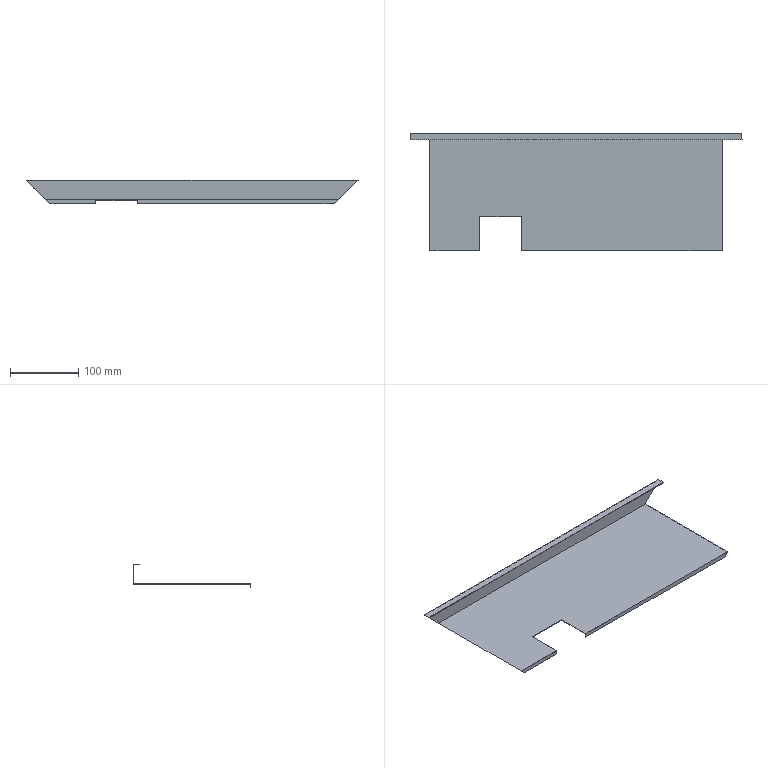Part | STEP file | 09-07 Inner side plate 4 | 1 solid | 18 faces | box 485 x 172 x 35 mm | volume 89624 mm3 | plane 18
STEP:
#1=CARTESIAN_POINT('',(0.,0.,0.));
#2=DIRECTION('',(0.,0.,1.));
#3=DIRECTION('',(1.,0.,0.));
#4=AXIS2_PLACEMENT_3D('',#1,#2,#3);
#5=CARTESIAN_POINT('',(162.5,50.,1.));
#6=VERTEX_POINT('',#5);
#7=CARTESIAN_POINT('',(102.,50.,1.));
#8=VERTEX_POINT('',#7);
#9=CARTESIAN_POINT('',(242.5,50.,1.));
#10=DIRECTION('',(-1.,0.,0.));
#11=VECTOR('',#10,1.);
#12=LINE('',#9,#11);
#13=CARTESIAN_POINT('',(29.,0.,1.));
#14=DIRECTION('',(0.,0.,-1.));
#15=DIRECTION('',(0.,1.,0.));
#16=AXIS2_PLACEMENT_3D('',#13,#14,#15);
#17=PLANE('',#16);
#18=CARTESIAN_POINT('',(50.,213.5));
#19=DIRECTION('',(0.,-1.));
#20=VECTOR('',#19,1.);
#21=LINE('',#18,#20);
#22=(GEOMETRIC_REPRESENTATION_CONTEXT(2)PARAMETRIC_REPRESENTATION_CONTEXT()REPRESENTATION_CONTEXT('',''));
#23=DEFINITIONAL_REPRESENTATION('',(#21),#22);
#24=PCURVE('',#17,#23);
#25=CARTESIAN_POINT('',(102.,50.,1.));
#26=DIRECTION('',(0.,-1.,0.));
#27=DIRECTION('',(0.,0.,-1.));
#28=AXIS2_PLACEMENT_3D('',#25,#26,#27);
#29=PLANE('',#28);
#30=CARTESIAN_POINT('',(0.,140.5));
#31=DIRECTION('',(0.,-1.));
#32=VECTOR('',#31,1.);
#33=LINE('',#30,#32);
#34=(GEOMETRIC_REPRESENTATION_CONTEXT(2)PARAMETRIC_REPRESENTATION_CONTEXT()REPRESENTATION_CONTEXT('',''));
#35=DEFINITIONAL_REPRESENTATION('',(#33),#34);
#36=PCURVE('',#29,#35);
#37=SURFACE_CURVE('',#12,(#24,#36),.PCURVE_S1.);
#38=EDGE_CURVE('',#6,#8,#37,.T.);
#39=ORIENTED_EDGE('',*,*,#38,.F.);
#40=CARTESIAN_POINT('',(162.5,0.,1.));
#41=VERTEX_POINT('',#40);
#42=CARTESIAN_POINT('',(162.5,85.5,1.));
#43=DIRECTION('',(0.,1.,0.));
#44=VECTOR('',#43,1.);
#45=LINE('',#42,#44);
#46=CARTESIAN_POINT('',(85.5,133.5));
#47=DIRECTION('',(1.,0.));
#48=VECTOR('',#47,1.);
#49=LINE('',#46,#48);
#50=(GEOMETRIC_REPRESENTATION_CONTEXT(2)PARAMETRIC_REPRESENTATION_CONTEXT()REPRESENTATION_CONTEXT('',''));
#51=DEFINITIONAL_REPRESENTATION('',(#49),#50);
#52=PCURVE('',#17,#51);
#53=CARTESIAN_POINT('',(162.5,0.,-5.));
#54=DIRECTION('',(-1.,0.,0.));
#55=DIRECTION('',(0.,0.,1.));
#56=AXIS2_PLACEMENT_3D('',#53,#54,#55);
#57=PLANE('',#56);
#58=CARTESIAN_POINT('',(6.,85.5));
#59=DIRECTION('',(0.,1.));
#60=VECTOR('',#59,1.);
#61=LINE('',#58,#60);
#62=(GEOMETRIC_REPRESENTATION_CONTEXT(2)PARAMETRIC_REPRESENTATION_CONTEXT()REPRESENTATION_CONTEXT('',''));
#63=DEFINITIONAL_REPRESENTATION('',(#61),#62);
#64=PCURVE('',#57,#63);
#65=SURFACE_CURVE('',#45,(#52,#64),.PCURVE_S1.);
#66=EDGE_CURVE('',#41,#6,#65,.T.);
#67=ORIENTED_EDGE('',*,*,#66,.F.);
#68=CARTESIAN_POINT('',(456.,0.,1.));
#69=VERTEX_POINT('',#68);
#70=CARTESIAN_POINT('',(242.5,0.,1.));
#71=DIRECTION('',(-1.,0.,0.));
#72=VECTOR('',#71,1.);
#73=LINE('',#70,#72);
#74=CARTESIAN_POINT('',(0.,213.5));
#75=DIRECTION('',(0.,-1.));
#76=VECTOR('',#75,1.);
#77=LINE('',#74,#76);
#78=(GEOMETRIC_REPRESENTATION_CONTEXT(2)PARAMETRIC_REPRESENTATION_CONTEXT()REPRESENTATION_CONTEXT('',''));
#79=DEFINITIONAL_REPRESENTATION('',(#77),#78);
#80=PCURVE('',#17,#79);
#81=CARTESIAN_POINT('',(162.5,0.,-5.));
#82=DIRECTION('',(0.,1.,0.));
#83=DIRECTION('',(0.,0.,1.));
#84=AXIS2_PLACEMENT_3D('',#81,#82,#83);
#85=PLANE('',#84);
#86=CARTESIAN_POINT('',(6.,80.));
#87=DIRECTION('',(0.,-1.));
#88=VECTOR('',#87,1.);
#89=LINE('',#86,#88);
#90=(GEOMETRIC_REPRESENTATION_CONTEXT(2)PARAMETRIC_REPRESENTATION_CONTEXT()REPRESENTATION_CONTEXT('',''));
#91=DEFINITIONAL_REPRESENTATION('',(#89),#90);
#92=PCURVE('',#85,#91);
#93=SURFACE_CURVE('',#73,(#80,#92),.PCURVE_S1.);
#94=EDGE_CURVE('',#69,#41,#93,.T.);
#95=ORIENTED_EDGE('',*,*,#94,.F.);
#96=CARTESIAN_POINT('',(456.,171.,1.));
#97=VERTEX_POINT('',#96);
#98=CARTESIAN_POINT('',(456.,85.5,1.));
#99=DIRECTION('',(0.,-1.,0.));
#100=VECTOR('',#99,1.);
#101=LINE('',#98,#100);
#102=CARTESIAN_POINT('',(85.5,427.));
#103=DIRECTION('',(-1.,0.));
#104=VECTOR('',#103,1.);
#105=LINE('',#102,#104);
#106=(GEOMETRIC_REPRESENTATION_CONTEXT(2)PARAMETRIC_REPRESENTATION_CONTEXT()REPRESENTATION_CONTEXT('',''));
#107=DEFINITIONAL_REPRESENTATION('',(#105),#106);
#108=PCURVE('',#17,#107);
#109=CARTESIAN_POINT('',(450.,0.,-5.));
#110=DIRECTION('',(-0.7071,0.,0.7071));
#111=DIRECTION('',(0.7071,0.,0.7071));
#112=AXIS2_PLACEMENT_3D('',#109,#110,#111);
#113=PLANE('',#112);
#114=CARTESIAN_POINT('',(8.485,85.5));
#115=DIRECTION('',(0.,-1.));
#116=VECTOR('',#115,1.);
#117=LINE('',#114,#116);
#118=(GEOMETRIC_REPRESENTATION_CONTEXT(2)PARAMETRIC_REPRESENTATION_CONTEXT()REPRESENTATION_CONTEXT('',''));
#119=DEFINITIONAL_REPRESENTATION('',(#117),#118);
#120=PCURVE('',#113,#119);
#121=SURFACE_CURVE('',#101,(#108,#120),.PCURVE_S1.);
#122=EDGE_CURVE('',#97,#69,#121,.T.);
#123=ORIENTED_EDGE('',*,*,#122,.F.);
#124=CARTESIAN_POINT('',(29.,171.,1.));
#125=VERTEX_POINT('',#124);
#126=CARTESIAN_POINT('',(242.5,171.,1.));
#127=DIRECTION('',(1.,0.,0.));
#128=VECTOR('',#127,1.);
#129=LINE('',#126,#128);
#130=CARTESIAN_POINT('',(171.,213.5));
#131=DIRECTION('',(0.,1.));
#132=VECTOR('',#131,1.);
#133=LINE('',#130,#132);
#134=(GEOMETRIC_REPRESENTATION_CONTEXT(2)PARAMETRIC_REPRESENTATION_CONTEXT()REPRESENTATION_CONTEXT('',''));
#135=DEFINITIONAL_REPRESENTATION('',(#133),#134);
#136=PCURVE('',#17,#135);
#137=CARTESIAN_POINT('',(-1.898,171.,1.));
#138=DIRECTION('',(0.,1.,0.));
#139=DIRECTION('',(0.,0.,1.));
#140=AXIS2_PLACEMENT_3D('',#137,#138,#139);
#141=PLANE('',#140);
#142=CARTESIAN_POINT('',(0.,244.398));
#143=DIRECTION('',(0.,1.));
#144=VECTOR('',#143,1.);
#145=LINE('',#142,#144);
#146=(GEOMETRIC_REPRESENTATION_CONTEXT(2)PARAMETRIC_REPRESENTATION_CONTEXT()REPRESENTATION_CONTEXT('',''));
#147=DEFINITIONAL_REPRESENTATION('',(#145),#146);
#148=PCURVE('',#141,#147);
#149=SURFACE_CURVE('',#129,(#136,#148),.PCURVE_S1.);
#150=EDGE_CURVE('',#125,#97,#149,.T.);
#151=ORIENTED_EDGE('',*,*,#150,.F.);
#152=CARTESIAN_POINT('',(29.,0.,1.));
#153=VERTEX_POINT('',#152);
#154=CARTESIAN_POINT('',(29.,85.5,1.));
#155=DIRECTION('',(0.,1.,0.));
#156=VECTOR('',#155,1.);
#157=LINE('',#154,#156);
#158=CARTESIAN_POINT('',(85.5,0.));
#159=DIRECTION('',(1.,0.));
#160=VECTOR('',#159,1.);
#161=LINE('',#158,#160);
#162=(GEOMETRIC_REPRESENTATION_CONTEXT(2)PARAMETRIC_REPRESENTATION_CONTEXT()REPRESENTATION_CONTEXT('',''));
#163=DEFINITIONAL_REPRESENTATION('',(#161),#162);
#164=PCURVE('',#17,#163);
#165=CARTESIAN_POINT('',(0.,0.,30.));
#166=DIRECTION('',(0.7071,0.,0.7071));
#167=DIRECTION('',(0.7071,0.,-0.7071));
#168=AXIS2_PLACEMENT_3D('',#165,#166,#167);
#169=PLANE('',#168);
#170=CARTESIAN_POINT('',(41.012,85.5));
#171=DIRECTION('',(0.,1.));
#172=VECTOR('',#171,1.);
#173=LINE('',#170,#172);
#174=(GEOMETRIC_REPRESENTATION_CONTEXT(2)PARAMETRIC_REPRESENTATION_CONTEXT()REPRESENTATION_CONTEXT('',''));
#175=DEFINITIONAL_REPRESENTATION('',(#173),#174);
#176=PCURVE('',#169,#175);
#177=SURFACE_CURVE('',#157,(#164,#176),.PCURVE_S1.);
#178=EDGE_CURVE('',#153,#125,#177,.T.);
#179=ORIENTED_EDGE('',*,*,#178,.F.);
#180=CARTESIAN_POINT('',(102.,0.,1.));
#181=VERTEX_POINT('',#180);
#182=CARTESIAN_POINT('',(242.5,0.,1.));
#183=DIRECTION('',(-1.,0.,0.));
#184=VECTOR('',#183,1.);
#185=LINE('',#182,#184);
#186=CARTESIAN_POINT('',(0.,213.5));
#187=DIRECTION('',(0.,-1.));
#188=VECTOR('',#187,1.);
#189=LINE('',#186,#188);
#190=(GEOMETRIC_REPRESENTATION_CONTEXT(2)PARAMETRIC_REPRESENTATION_CONTEXT()REPRESENTATION_CONTEXT('',''));
#191=DEFINITIONAL_REPRESENTATION('',(#189),#190);
#192=PCURVE('',#17,#191);
#193=CARTESIAN_POINT('',(28.562,0.,-5.));
#194=DIRECTION('',(0.,1.,0.));
#195=DIRECTION('',(0.,0.,1.));
#196=AXIS2_PLACEMENT_3D('',#193,#194,#195);
#197=PLANE('',#196);
#198=CARTESIAN_POINT('',(6.,213.938));
#199=DIRECTION('',(0.,-1.));
#200=VECTOR('',#199,1.);
#201=LINE('',#198,#200);
#202=(GEOMETRIC_REPRESENTATION_CONTEXT(2)PARAMETRIC_REPRESENTATION_CONTEXT()REPRESENTATION_CONTEXT('',''));
#203=DEFINITIONAL_REPRESENTATION('',(#201),#202);
#204=PCURVE('',#197,#203);
#205=SURFACE_CURVE('',#185,(#192,#204),.PCURVE_S1.);
#206=EDGE_CURVE('',#181,#153,#205,.T.);
#207=ORIENTED_EDGE('',*,*,#206,.F.);
#208=CARTESIAN_POINT('',(102.,85.5,1.));
#209=DIRECTION('',(0.,-1.,0.));
#210=VECTOR('',#209,1.);
#211=LINE('',#208,#210);
#212=CARTESIAN_POINT('',(85.5,73.));
#213=DIRECTION('',(-1.,0.));
#214=VECTOR('',#213,1.);
#215=LINE('',#212,#214);
#216=(GEOMETRIC_REPRESENTATION_CONTEXT(2)PARAMETRIC_REPRESENTATION_CONTEXT()REPRESENTATION_CONTEXT('',''));
#217=DEFINITIONAL_REPRESENTATION('',(#215),#216);
#218=PCURVE('',#17,#217);
#219=CARTESIAN_POINT('',(102.,0.,-5.));
#220=DIRECTION('',(1.,0.,0.));
#221=DIRECTION('',(0.,1.,0.));
#222=AXIS2_PLACEMENT_3D('',#219,#220,#221);
#223=PLANE('',#222);
#224=CARTESIAN_POINT('',(85.5,6.));
#225=DIRECTION('',(-1.,0.));
#226=VECTOR('',#225,1.);
#227=LINE('',#224,#226);
#228=(GEOMETRIC_REPRESENTATION_CONTEXT(2)PARAMETRIC_REPRESENTATION_CONTEXT()REPRESENTATION_CONTEXT('',''));
#229=DEFINITIONAL_REPRESENTATION('',(#227),#228);
#230=PCURVE('',#223,#229);
#231=SURFACE_CURVE('',#211,(#218,#230),.PCURVE_S1.);
#232=EDGE_CURVE('',#8,#181,#231,.T.);
#233=ORIENTED_EDGE('',*,*,#232,.F.);
#234=EDGE_LOOP('',(#39,#67,#95,#123,#151,#179,#207,#233));
#235=FACE_BOUND('',#234,.T.);
#236=ADVANCED_FACE('',(#235),#17,.F.);
#237=CARTESIAN_POINT('',(102.,1.,-0.000000001));
#238=VERTEX_POINT('',#237);
#239=CARTESIAN_POINT('',(102.,50.,-0.000000001));
#240=VERTEX_POINT('',#239);
#241=CARTESIAN_POINT('',(102.,25.,-0.000000002));
#242=DIRECTION('',(0.,1.,0.));
#243=VECTOR('',#242,1.);
#244=LINE('',#241,#243);
#245=CARTESIAN_POINT('',(25.,5.));
#246=DIRECTION('',(1.,0.));
#247=VECTOR('',#246,1.);
#248=LINE('',#245,#247);
#249=(GEOMETRIC_REPRESENTATION_CONTEXT(2)PARAMETRIC_REPRESENTATION_CONTEXT()REPRESENTATION_CONTEXT('',''));
#250=DEFINITIONAL_REPRESENTATION('',(#248),#249);
#251=PCURVE('',#223,#250);
#252=CARTESIAN_POINT('',(30.,172.,0.));
#253=DIRECTION('',(0.,0.,1.));
#254=DIRECTION('',(0.,-1.,0.));
#255=AXIS2_PLACEMENT_3D('',#252,#253,#254);
#256=PLANE('',#255);
#257=CARTESIAN_POINT('',(147.,72.));
#258=DIRECTION('',(-1.,0.));
#259=VECTOR('',#258,1.);
#260=LINE('',#257,#259);
#261=(GEOMETRIC_REPRESENTATION_CONTEXT(2)PARAMETRIC_REPRESENTATION_CONTEXT()REPRESENTATION_CONTEXT('',''));
#262=DEFINITIONAL_REPRESENTATION('',(#260),#261);
#263=PCURVE('',#256,#262);
#264=SURFACE_CURVE('',#244,(#251,#263),.PCURVE_S1.);
#265=EDGE_CURVE('',#238,#240,#264,.T.);
#266=ORIENTED_EDGE('',*,*,#265,.T.);
#267=CARTESIAN_POINT('',(102.,50.,-2.));
#268=DIRECTION('',(0.,0.,1.));
#269=VECTOR('',#268,1.);
#270=LINE('',#267,#269);
#271=CARTESIAN_POINT('',(50.,3.));
#272=DIRECTION('',(0.,1.));
#273=VECTOR('',#272,1.);
#274=LINE('',#271,#273);
#275=(GEOMETRIC_REPRESENTATION_CONTEXT(2)PARAMETRIC_REPRESENTATION_CONTEXT()REPRESENTATION_CONTEXT('',''));
#276=DEFINITIONAL_REPRESENTATION('',(#274),#275);
#277=PCURVE('',#223,#276);
#278=CARTESIAN_POINT('',(3.,0.));
#279=DIRECTION('',(-1.,0.));
#280=VECTOR('',#279,1.);
#281=LINE('',#278,#280);
#282=(GEOMETRIC_REPRESENTATION_CONTEXT(2)PARAMETRIC_REPRESENTATION_CONTEXT()REPRESENTATION_CONTEXT('',''));
#283=DEFINITIONAL_REPRESENTATION('',(#281),#282);
#284=PCURVE('',#29,#283);
#285=SURFACE_CURVE('',#270,(#277,#284),.PCURVE_S1.);
#286=EDGE_CURVE('',#240,#8,#285,.T.);
#287=ORIENTED_EDGE('',*,*,#286,.T.);
#288=ORIENTED_EDGE('',*,*,#232,.T.);
#289=CARTESIAN_POINT('',(102.,0.,-5.));
#290=VERTEX_POINT('',#289);
#291=CARTESIAN_POINT('',(102.,0.,-2.));
#292=DIRECTION('',(0.,0.,-1.));
#293=VECTOR('',#292,1.);
#294=LINE('',#291,#293);
#295=CARTESIAN_POINT('',(0.,3.));
#296=DIRECTION('',(0.,-1.));
#297=VECTOR('',#296,1.);
#298=LINE('',#295,#297);
#299=(GEOMETRIC_REPRESENTATION_CONTEXT(2)PARAMETRIC_REPRESENTATION_CONTEXT()REPRESENTATION_CONTEXT('',''));
#300=DEFINITIONAL_REPRESENTATION('',(#298),#299);
#301=PCURVE('',#223,#300);
#302=CARTESIAN_POINT('',(3.,73.438));
#303=DIRECTION('',(-1.,0.));
#304=VECTOR('',#303,1.);
#305=LINE('',#302,#304);
#306=(GEOMETRIC_REPRESENTATION_CONTEXT(2)PARAMETRIC_REPRESENTATION_CONTEXT()REPRESENTATION_CONTEXT('',''));
#307=DEFINITIONAL_REPRESENTATION('',(#305),#306);
#308=PCURVE('',#197,#307);
#309=SURFACE_CURVE('',#294,(#301,#308),.PCURVE_S1.);
#310=EDGE_CURVE('',#181,#290,#309,.T.);
#311=ORIENTED_EDGE('',*,*,#310,.T.);
#312=CARTESIAN_POINT('',(102.,1.,-5.));
#313=VERTEX_POINT('',#312);
#314=CARTESIAN_POINT('',(102.,0.5,-5.));
#315=DIRECTION('',(0.,1.,0.));
#316=VECTOR('',#315,1.);
#317=LINE('',#314,#316);
#318=CARTESIAN_POINT('',(0.5,0.));
#319=DIRECTION('',(1.,0.));
#320=VECTOR('',#319,1.);
#321=LINE('',#318,#320);
#322=(GEOMETRIC_REPRESENTATION_CONTEXT(2)PARAMETRIC_REPRESENTATION_CONTEXT()REPRESENTATION_CONTEXT('',''));
#323=DEFINITIONAL_REPRESENTATION('',(#321),#322);
#324=PCURVE('',#223,#323);
#325=CARTESIAN_POINT('',(35.,0.,-5.));
#326=DIRECTION('',(0.,0.,1.));
#327=DIRECTION('',(1.,0.,0.));
#328=AXIS2_PLACEMENT_3D('',#325,#326,#327);
#329=PLANE('',#328);
#330=CARTESIAN_POINT('',(67.,0.5));
#331=DIRECTION('',(0.,1.));
#332=VECTOR('',#331,1.);
#333=LINE('',#330,#332);
#334=(GEOMETRIC_REPRESENTATION_CONTEXT(2)PARAMETRIC_REPRESENTATION_CONTEXT()REPRESENTATION_CONTEXT('',''));
#335=DEFINITIONAL_REPRESENTATION('',(#333),#334);
#336=PCURVE('',#329,#335);
#337=SURFACE_CURVE('',#317,(#324,#336),.PCURVE_S1.);
#338=EDGE_CURVE('',#290,#313,#337,.T.);
#339=ORIENTED_EDGE('',*,*,#338,.T.);
#340=CARTESIAN_POINT('',(102.,1.,-2.));
#341=DIRECTION('',(0.,0.,1.));
#342=VECTOR('',#341,1.);
#343=LINE('',#340,#342);
#344=CARTESIAN_POINT('',(1.,3.));
#345=DIRECTION('',(0.,1.));
#346=VECTOR('',#345,1.);
#347=LINE('',#344,#346);
#348=(GEOMETRIC_REPRESENTATION_CONTEXT(2)PARAMETRIC_REPRESENTATION_CONTEXT()REPRESENTATION_CONTEXT('',''));
#349=DEFINITIONAL_REPRESENTATION('',(#347),#348);
#350=PCURVE('',#223,#349);
#351=CARTESIAN_POINT('',(29.568,1.,0.));
#352=DIRECTION('',(0.,-1.,0.));
#353=DIRECTION('',(0.,0.,-1.));
#354=AXIS2_PLACEMENT_3D('',#351,#352,#353);
#355=PLANE('',#354);
#356=CARTESIAN_POINT('',(2.,72.432));
#357=DIRECTION('',(-1.,0.));
#358=VECTOR('',#357,1.);
#359=LINE('',#356,#358);
#360=(GEOMETRIC_REPRESENTATION_CONTEXT(2)PARAMETRIC_REPRESENTATION_CONTEXT()REPRESENTATION_CONTEXT('',''));
#361=DEFINITIONAL_REPRESENTATION('',(#359),#360);
#362=PCURVE('',#355,#361);
#363=SURFACE_CURVE('',#343,(#350,#362),.PCURVE_S1.);
#364=EDGE_CURVE('',#313,#238,#363,.T.);
#365=ORIENTED_EDGE('',*,*,#364,.T.);
#366=EDGE_LOOP('',(#266,#287,#288,#311,#339,#365));
#367=FACE_BOUND('',#366,.T.);
#368=ADVANCED_FACE('',(#367),#223,.T.);
#369=CARTESIAN_POINT('',(162.5,50.,-0.000000001));
#370=VERTEX_POINT('',#369);
#371=CARTESIAN_POINT('',(132.25,50.,0.));
#372=DIRECTION('',(1.,0.,0.));
#373=VECTOR('',#372,1.);
#374=LINE('',#371,#373);
#375=CARTESIAN_POINT('',(1.,30.25));
#376=DIRECTION('',(0.,1.));
#377=VECTOR('',#376,1.);
#378=LINE('',#375,#377);
#379=(GEOMETRIC_REPRESENTATION_CONTEXT(2)PARAMETRIC_REPRESENTATION_CONTEXT()REPRESENTATION_CONTEXT('',''));
#380=DEFINITIONAL_REPRESENTATION('',(#378),#379);
#381=PCURVE('',#29,#380);
#382=CARTESIAN_POINT('',(122.,102.25));
#383=DIRECTION('',(0.,1.));
#384=VECTOR('',#383,1.);
#385=LINE('',#382,#384);
#386=(GEOMETRIC_REPRESENTATION_CONTEXT(2)PARAMETRIC_REPRESENTATION_CONTEXT()REPRESENTATION_CONTEXT('',''));
#387=DEFINITIONAL_REPRESENTATION('',(#385),#386);
#388=PCURVE('',#256,#387);
#389=SURFACE_CURVE('',#374,(#381,#388),.PCURVE_S1.);
#390=EDGE_CURVE('',#240,#370,#389,.T.);
#391=ORIENTED_EDGE('',*,*,#390,.T.);
#392=CARTESIAN_POINT('',(162.5,50.,0.5));
#393=DIRECTION('',(0.,0.,1.));
#394=VECTOR('',#393,1.);
#395=LINE('',#392,#394);
#396=CARTESIAN_POINT('',(0.5,60.5));
#397=DIRECTION('',(-1.,0.));
#398=VECTOR('',#397,1.);
#399=LINE('',#396,#398);
#400=(GEOMETRIC_REPRESENTATION_CONTEXT(2)PARAMETRIC_REPRESENTATION_CONTEXT()REPRESENTATION_CONTEXT('',''));
#401=DEFINITIONAL_REPRESENTATION('',(#399),#400);
#402=PCURVE('',#29,#401);
#403=CARTESIAN_POINT('',(5.5,50.));
#404=DIRECTION('',(1.,0.));
#405=VECTOR('',#404,1.);
#406=LINE('',#403,#405);
#407=(GEOMETRIC_REPRESENTATION_CONTEXT(2)PARAMETRIC_REPRESENTATION_CONTEXT()REPRESENTATION_CONTEXT('',''));
#408=DEFINITIONAL_REPRESENTATION('',(#406),#407);
#409=PCURVE('',#57,#408);
#410=SURFACE_CURVE('',#395,(#402,#409),.PCURVE_S1.);
#411=EDGE_CURVE('',#370,#6,#410,.T.);
#412=ORIENTED_EDGE('',*,*,#411,.T.);
#413=ORIENTED_EDGE('',*,*,#38,.T.);
#414=ORIENTED_EDGE('',*,*,#286,.F.);
#415=EDGE_LOOP('',(#391,#412,#413,#414));
#416=FACE_BOUND('',#415,.T.);
#417=ADVANCED_FACE('',(#416),#29,.T.);
#418=CARTESIAN_POINT('',(162.5,1.,-5.));
#419=VERTEX_POINT('',#418);
#420=CARTESIAN_POINT('',(162.5,0.,-5.));
#421=VERTEX_POINT('',#420);
#422=CARTESIAN_POINT('',(162.5,0.5,-5.));
#423=DIRECTION('',(0.,-1.,0.));
#424=VECTOR('',#423,1.);
#425=LINE('',#422,#424);
#426=CARTESIAN_POINT('',(0.,0.5));
#427=DIRECTION('',(0.,-1.));
#428=VECTOR('',#427,1.);
#429=LINE('',#426,#428);
#430=(GEOMETRIC_REPRESENTATION_CONTEXT(2)PARAMETRIC_REPRESENTATION_CONTEXT()REPRESENTATION_CONTEXT('',''));
#431=DEFINITIONAL_REPRESENTATION('',(#429),#430);
#432=PCURVE('',#57,#431);
#433=CARTESIAN_POINT('',(162.5,0.,-5.));
#434=DIRECTION('',(0.,0.,1.));
#435=DIRECTION('',(1.,0.,0.));
#436=AXIS2_PLACEMENT_3D('',#433,#434,#435);
#437=PLANE('',#436);
#438=CARTESIAN_POINT('',(0.,0.5));
#439=DIRECTION('',(0.,-1.));
#440=VECTOR('',#439,1.);
#441=LINE('',#438,#440);
#442=(GEOMETRIC_REPRESENTATION_CONTEXT(2)PARAMETRIC_REPRESENTATION_CONTEXT()REPRESENTATION_CONTEXT('',''));
#443=DEFINITIONAL_REPRESENTATION('',(#441),#442);
#444=PCURVE('',#437,#443);
#445=SURFACE_CURVE('',#425,(#432,#444),.PCURVE_S1.);
#446=EDGE_CURVE('',#419,#421,#445,.T.);
#447=ORIENTED_EDGE('',*,*,#446,.T.);
#448=CARTESIAN_POINT('',(162.5,0.,-2.));
#449=DIRECTION('',(0.,0.,1.));
#450=VECTOR('',#449,1.);
#451=LINE('',#448,#450);
#452=CARTESIAN_POINT('',(3.,0.));
#453=DIRECTION('',(1.,0.));
#454=VECTOR('',#453,1.);
#455=LINE('',#452,#454);
#456=(GEOMETRIC_REPRESENTATION_CONTEXT(2)PARAMETRIC_REPRESENTATION_CONTEXT()REPRESENTATION_CONTEXT('',''));
#457=DEFINITIONAL_REPRESENTATION('',(#455),#456);
#458=PCURVE('',#57,#457);
#459=CARTESIAN_POINT('',(3.,0.));
#460=DIRECTION('',(1.,0.));
#461=VECTOR('',#460,1.);
#462=LINE('',#459,#461);
#463=(GEOMETRIC_REPRESENTATION_CONTEXT(2)PARAMETRIC_REPRESENTATION_CONTEXT()REPRESENTATION_CONTEXT('',''));
#464=DEFINITIONAL_REPRESENTATION('',(#462),#463);
#465=PCURVE('',#85,#464);
#466=SURFACE_CURVE('',#451,(#458,#465),.PCURVE_S1.);
#467=EDGE_CURVE('',#421,#41,#466,.T.);
#468=ORIENTED_EDGE('',*,*,#467,.T.);
#469=ORIENTED_EDGE('',*,*,#66,.T.);
#470=ORIENTED_EDGE('',*,*,#411,.F.);
#471=CARTESIAN_POINT('',(162.5,1.,-0.000000001));
#472=VERTEX_POINT('',#471);
#473=CARTESIAN_POINT('',(162.5,25.,-0.000000002));
#474=DIRECTION('',(0.,-1.,0.));
#475=VECTOR('',#474,1.);
#476=LINE('',#473,#475);
#477=CARTESIAN_POINT('',(5.,25.));
#478=DIRECTION('',(0.,-1.));
#479=VECTOR('',#478,1.);
#480=LINE('',#477,#479);
#481=(GEOMETRIC_REPRESENTATION_CONTEXT(2)PARAMETRIC_REPRESENTATION_CONTEXT()REPRESENTATION_CONTEXT('',''));
#482=DEFINITIONAL_REPRESENTATION('',(#480),#481);
#483=PCURVE('',#57,#482);
#484=CARTESIAN_POINT('',(147.,132.5));
#485=DIRECTION('',(1.,0.));
#486=VECTOR('',#485,1.);
#487=LINE('',#484,#486);
#488=(GEOMETRIC_REPRESENTATION_CONTEXT(2)PARAMETRIC_REPRESENTATION_CONTEXT()REPRESENTATION_CONTEXT('',''));
#489=DEFINITIONAL_REPRESENTATION('',(#487),#488);
#490=PCURVE('',#256,#489);
#491=SURFACE_CURVE('',#476,(#483,#490),.PCURVE_S1.);
#492=EDGE_CURVE('',#370,#472,#491,.T.);
#493=ORIENTED_EDGE('',*,*,#492,.T.);
#494=CARTESIAN_POINT('',(162.5,1.,-2.));
#495=DIRECTION('',(0.,0.,-1.));
#496=VECTOR('',#495,1.);
#497=LINE('',#494,#496);
#498=CARTESIAN_POINT('',(3.,1.));
#499=DIRECTION('',(-1.,0.));
#500=VECTOR('',#499,1.);
#501=LINE('',#498,#500);
#502=(GEOMETRIC_REPRESENTATION_CONTEXT(2)PARAMETRIC_REPRESENTATION_CONTEXT()REPRESENTATION_CONTEXT('',''));
#503=DEFINITIONAL_REPRESENTATION('',(#501),#502);
#504=PCURVE('',#57,#503);
#505=CARTESIAN_POINT('',(162.5,1.,0.));
#506=DIRECTION('',(0.,-1.,0.));
#507=DIRECTION('',(0.,0.,-1.));
#508=AXIS2_PLACEMENT_3D('',#505,#506,#507);
#509=PLANE('',#508);
#510=CARTESIAN_POINT('',(2.,0.));
#511=DIRECTION('',(1.,0.));
#512=VECTOR('',#511,1.);
#513=LINE('',#510,#512);
#514=(GEOMETRIC_REPRESENTATION_CONTEXT(2)PARAMETRIC_REPRESENTATION_CONTEXT()REPRESENTATION_CONTEXT('',''));
#515=DEFINITIONAL_REPRESENTATION('',(#513),#514);
#516=PCURVE('',#509,#515);
#517=SURFACE_CURVE('',#497,(#504,#516),.PCURVE_S1.);
#518=EDGE_CURVE('',#472,#419,#517,.T.);
#519=ORIENTED_EDGE('',*,*,#518,.T.);
#520=EDGE_LOOP('',(#447,#468,#469,#470,#493,#519));
#521=FACE_BOUND('',#520,.T.);
#522=ADVANCED_FACE('',(#521),#57,.T.);
#523=CARTESIAN_POINT('',(450.,0.,-5.));
#524=VERTEX_POINT('',#523);
#525=CARTESIAN_POINT('',(310.13,0.,-5.));
#526=DIRECTION('',(-1.,0.,0.));
#527=VECTOR('',#526,1.);
#528=LINE('',#525,#527);
#529=CARTESIAN_POINT('',(0.,147.631));
#530=DIRECTION('',(0.,-1.));
#531=VECTOR('',#530,1.);
#532=LINE('',#529,#531);
#533=(GEOMETRIC_REPRESENTATION_CONTEXT(2)PARAMETRIC_REPRESENTATION_CONTEXT()REPRESENTATION_CONTEXT('',''));
#534=DEFINITIONAL_REPRESENTATION('',(#532),#533);
#535=PCURVE('',#85,#534);
#536=CARTESIAN_POINT('',(147.631,0.));
#537=DIRECTION('',(-1.,0.));
#538=VECTOR('',#537,1.);
#539=LINE('',#536,#538);
#540=(GEOMETRIC_REPRESENTATION_CONTEXT(2)PARAMETRIC_REPRESENTATION_CONTEXT()REPRESENTATION_CONTEXT('',''));
#541=DEFINITIONAL_REPRESENTATION('',(#539),#540);
#542=PCURVE('',#437,#541);
#543=SURFACE_CURVE('',#528,(#535,#542),.PCURVE_S1.);
#544=EDGE_CURVE('',#524,#421,#543,.T.);
#545=ORIENTED_EDGE('',*,*,#544,.F.);
#546=CARTESIAN_POINT('',(450.,0.,-5.));
#547=DIRECTION('',(-0.7071,0.,-0.7071));
#548=VECTOR('',#547,1.);
#549=LINE('',#546,#548);
#550=CARTESIAN_POINT('',(0.,287.5));
#551=DIRECTION('',(-0.7071,-0.7071));
#552=VECTOR('',#551,1.);
#553=LINE('',#550,#552);
#554=(GEOMETRIC_REPRESENTATION_CONTEXT(2)PARAMETRIC_REPRESENTATION_CONTEXT()REPRESENTATION_CONTEXT('',''));
#555=DEFINITIONAL_REPRESENTATION('',(#553),#554);
#556=PCURVE('',#85,#555);
#557=CARTESIAN_POINT('',(0.,0.));
#558=DIRECTION('',(-1.,0.));
#559=VECTOR('',#558,1.);
#560=LINE('',#557,#559);
#561=(GEOMETRIC_REPRESENTATION_CONTEXT(2)PARAMETRIC_REPRESENTATION_CONTEXT()REPRESENTATION_CONTEXT('',''));
#562=DEFINITIONAL_REPRESENTATION('',(#560),#561);
#563=PCURVE('',#113,#562);
#564=SURFACE_CURVE('',#549,(#556,#563),.PCURVE_S1.);
#565=EDGE_CURVE('',#69,#524,#564,.T.);
#566=ORIENTED_EDGE('',*,*,#565,.F.);
#567=ORIENTED_EDGE('',*,*,#94,.T.);
#568=ORIENTED_EDGE('',*,*,#467,.F.);
#569=EDGE_LOOP('',(#545,#566,#567,#568));
#570=FACE_BOUND('',#569,.T.);
#571=ADVANCED_FACE('',(#570),#85,.F.);
#572=CARTESIAN_POINT('',(485.,172.,30.));
#573=VERTEX_POINT('',#572);
#574=CARTESIAN_POINT('',(455.,172.,0.000000001));
#575=VERTEX_POINT('',#574);
#576=CARTESIAN_POINT('',(467.5,172.,12.5));
#577=DIRECTION('',(-0.7071,0.,-0.7071));
#578=VECTOR('',#577,1.);
#579=LINE('',#576,#578);
#580=CARTESIAN_POINT('',(24.749,172.));
#581=DIRECTION('',(-1.,0.));
#582=VECTOR('',#581,1.);
#583=LINE('',#580,#582);
#584=(GEOMETRIC_REPRESENTATION_CONTEXT(2)PARAMETRIC_REPRESENTATION_CONTEXT()REPRESENTATION_CONTEXT('',''));
#585=DEFINITIONAL_REPRESENTATION('',(#583),#584);
#586=PCURVE('',#113,#585);
#587=CARTESIAN_POINT('',(-2.91,172.,30.));
#588=DIRECTION('',(0.,-1.,0.));
#589=DIRECTION('',(0.,0.,-1.));
#590=AXIS2_PLACEMENT_3D('',#587,#588,#589);
#591=PLANE('',#590);
#592=CARTESIAN_POINT('',(17.5,470.41));
#593=DIRECTION('',(0.7071,-0.7071));
#594=VECTOR('',#593,1.);
#595=LINE('',#592,#594);
#596=(GEOMETRIC_REPRESENTATION_CONTEXT(2)PARAMETRIC_REPRESENTATION_CONTEXT()REPRESENTATION_CONTEXT('',''));
#597=DEFINITIONAL_REPRESENTATION('',(#595),#596);
#598=PCURVE('',#591,#597);
#599=SURFACE_CURVE('',#579,(#586,#598),.PCURVE_S1.);
#600=EDGE_CURVE('',#573,#575,#599,.T.);
#601=ORIENTED_EDGE('',*,*,#600,.F.);
#602=CARTESIAN_POINT('',(485.,162.,30.));
#603=VERTEX_POINT('',#602);
#604=CARTESIAN_POINT('',(485.,86.,30.));
#605=DIRECTION('',(0.,1.,0.));
#606=VECTOR('',#605,1.);
#607=LINE('',#604,#606);
#608=CARTESIAN_POINT('',(49.497,86.));
#609=DIRECTION('',(0.,1.));
#610=VECTOR('',#609,1.);
#611=LINE('',#608,#610);
#612=(GEOMETRIC_REPRESENTATION_CONTEXT(2)PARAMETRIC_REPRESENTATION_CONTEXT()REPRESENTATION_CONTEXT('',''));
#613=DEFINITIONAL_REPRESENTATION('',(#611),#612);
#614=PCURVE('',#113,#613);
#615=CARTESIAN_POINT('',(0.,162.,30.));
#616=DIRECTION('',(0.,0.,-1.));
#617=DIRECTION('',(0.,1.,0.));
#618=AXIS2_PLACEMENT_3D('',#615,#616,#617);
#619=PLANE('',#618);
#620=CARTESIAN_POINT('',(-76.,485.));
#621=DIRECTION('',(1.,0.));
#622=VECTOR('',#621,1.);
#623=LINE('',#620,#622);
#624=(GEOMETRIC_REPRESENTATION_CONTEXT(2)PARAMETRIC_REPRESENTATION_CONTEXT()REPRESENTATION_CONTEXT('',''));
#625=DEFINITIONAL_REPRESENTATION('',(#623),#624);
#626=PCURVE('',#619,#625);
#627=SURFACE_CURVE('',#607,(#614,#626),.PCURVE_S1.);
#628=EDGE_CURVE('',#603,#573,#627,.T.);
#629=ORIENTED_EDGE('',*,*,#628,.F.);
#630=CARTESIAN_POINT('',(484.,162.,29.));
#631=VERTEX_POINT('',#630);
#632=CARTESIAN_POINT('',(450.,162.,-5.));
#633=DIRECTION('',(-0.7071,0.,-0.7071));
#634=VECTOR('',#633,1.);
#635=LINE('',#632,#634);
#636=CARTESIAN_POINT('',(0.,162.));
#637=DIRECTION('',(-1.,0.));
#638=VECTOR('',#637,1.);
#639=LINE('',#636,#638);
#640=(GEOMETRIC_REPRESENTATION_CONTEXT(2)PARAMETRIC_REPRESENTATION_CONTEXT()REPRESENTATION_CONTEXT('',''));
#641=DEFINITIONAL_REPRESENTATION('',(#639),#640);
#642=PCURVE('',#113,#641);
#643=CARTESIAN_POINT('',(-2.91,162.,29.));
#644=DIRECTION('',(0.,1.,0.));
#645=DIRECTION('',(0.,0.,1.));
#646=AXIS2_PLACEMENT_3D('',#643,#644,#645);
#647=PLANE('',#646);
#648=CARTESIAN_POINT('',(-34.,452.91));
#649=DIRECTION('',(-0.7071,-0.7071));
#650=VECTOR('',#649,1.);
#651=LINE('',#648,#650);
#652=(GEOMETRIC_REPRESENTATION_CONTEXT(2)PARAMETRIC_REPRESENTATION_CONTEXT()REPRESENTATION_CONTEXT('',''));
#653=DEFINITIONAL_REPRESENTATION('',(#651),#652);
#654=PCURVE('',#647,#653);
#655=SURFACE_CURVE('',#635,(#642,#654),.PCURVE_S1.);
#656=EDGE_CURVE('',#603,#631,#655,.T.);
#657=ORIENTED_EDGE('',*,*,#656,.T.);
#658=CARTESIAN_POINT('',(484.,171.,29.));
#659=VERTEX_POINT('',#658);
#660=CARTESIAN_POINT('',(484.,86.,29.));
#661=DIRECTION('',(0.,-1.,0.));
#662=VECTOR('',#661,1.);
#663=LINE('',#660,#662);
#664=CARTESIAN_POINT('',(48.083,86.));
#665=DIRECTION('',(0.,-1.));
#666=VECTOR('',#665,1.);
#667=LINE('',#664,#666);
#668=(GEOMETRIC_REPRESENTATION_CONTEXT(2)PARAMETRIC_REPRESENTATION_CONTEXT()REPRESENTATION_CONTEXT('',''));
#669=DEFINITIONAL_REPRESENTATION('',(#667),#668);
#670=PCURVE('',#113,#669);
#671=CARTESIAN_POINT('',(1.,162.,29.));
#672=DIRECTION('',(0.,0.,1.));
#673=DIRECTION('',(1.,0.,0.));
#674=AXIS2_PLACEMENT_3D('',#671,#672,#673);
#675=PLANE('',#674);
#676=CARTESIAN_POINT('',(483.,-76.));
#677=DIRECTION('',(0.,-1.));
#678=VECTOR('',#677,1.);
#679=LINE('',#676,#678);
#680=(GEOMETRIC_REPRESENTATION_CONTEXT(2)PARAMETRIC_REPRESENTATION_CONTEXT()REPRESENTATION_CONTEXT('',''));
#681=DEFINITIONAL_REPRESENTATION('',(#679),#680);
#682=PCURVE('',#675,#681);
#683=SURFACE_CURVE('',#663,(#670,#682),.PCURVE_S1.);
#684=EDGE_CURVE('',#659,#631,#683,.T.);
#685=ORIENTED_EDGE('',*,*,#684,.F.);
#686=CARTESIAN_POINT('',(467.5,171.,12.5));
#687=DIRECTION('',(0.7071,0.,0.7071));
#688=VECTOR('',#687,1.);
#689=LINE('',#686,#688);
#690=CARTESIAN_POINT('',(24.749,171.));
#691=DIRECTION('',(1.,0.));
#692=VECTOR('',#691,1.);
#693=LINE('',#690,#692);
#694=(GEOMETRIC_REPRESENTATION_CONTEXT(2)PARAMETRIC_REPRESENTATION_CONTEXT()REPRESENTATION_CONTEXT('',''));
#695=DEFINITIONAL_REPRESENTATION('',(#693),#694);
#696=PCURVE('',#113,#695);
#697=CARTESIAN_POINT('',(11.5,469.398));
#698=DIRECTION('',(0.7071,0.7071));
#699=VECTOR('',#698,1.);
#700=LINE('',#697,#699);
#701=(GEOMETRIC_REPRESENTATION_CONTEXT(2)PARAMETRIC_REPRESENTATION_CONTEXT()REPRESENTATION_CONTEXT('',''));
#702=DEFINITIONAL_REPRESENTATION('',(#700),#701);
#703=PCURVE('',#141,#702);
#704=SURFACE_CURVE('',#689,(#696,#703),.PCURVE_S1.);
#705=EDGE_CURVE('',#97,#659,#704,.T.);
#706=ORIENTED_EDGE('',*,*,#705,.F.);
#707=ORIENTED_EDGE('',*,*,#122,.T.);
#708=ORIENTED_EDGE('',*,*,#565,.T.);
#709=CARTESIAN_POINT('',(450.,1.,-5.));
#710=VERTEX_POINT('',#709);
#711=CARTESIAN_POINT('',(450.,86.,-5.));
#712=DIRECTION('',(0.,-1.,0.));
#713=VECTOR('',#712,1.);
#714=LINE('',#711,#713);
#715=CARTESIAN_POINT('',(0.,86.));
#716=DIRECTION('',(0.,-1.));
#717=VECTOR('',#716,1.);
#718=LINE('',#715,#717);
#719=(GEOMETRIC_REPRESENTATION_CONTEXT(2)PARAMETRIC_REPRESENTATION_CONTEXT()REPRESENTATION_CONTEXT('',''));
#720=DEFINITIONAL_REPRESENTATION('',(#718),#719);
#721=PCURVE('',#113,#720);
#722=CARTESIAN_POINT('',(287.5,86.));
#723=DIRECTION('',(0.,-1.));
#724=VECTOR('',#723,1.);
#725=LINE('',#722,#724);
#726=(GEOMETRIC_REPRESENTATION_CONTEXT(2)PARAMETRIC_REPRESENTATION_CONTEXT()REPRESENTATION_CONTEXT('',''));
#727=DEFINITIONAL_REPRESENTATION('',(#725),#726);
#728=PCURVE('',#437,#727);
#729=SURFACE_CURVE('',#714,(#721,#728),.PCURVE_S1.);
#730=EDGE_CURVE('',#710,#524,#729,.T.);
#731=ORIENTED_EDGE('',*,*,#730,.F.);
#732=CARTESIAN_POINT('',(455.,1.,0.000000001));
#733=VERTEX_POINT('',#732);
#734=CARTESIAN_POINT('',(467.5,1.,12.5));
#735=DIRECTION('',(-0.7071,0.,-0.7071));
#736=VECTOR('',#735,1.);
#737=LINE('',#734,#736);
#738=CARTESIAN_POINT('',(24.749,1.));
#739=DIRECTION('',(-1.,0.));
#740=VECTOR('',#739,1.);
#741=LINE('',#738,#740);
#742=(GEOMETRIC_REPRESENTATION_CONTEXT(2)PARAMETRIC_REPRESENTATION_CONTEXT()REPRESENTATION_CONTEXT('',''));
#743=DEFINITIONAL_REPRESENTATION('',(#741),#742);
#744=PCURVE('',#113,#743);
#745=CARTESIAN_POINT('',(-12.5,305.));
#746=DIRECTION('',(0.7071,-0.7071));
#747=VECTOR('',#746,1.);
#748=LINE('',#745,#747);
#749=(GEOMETRIC_REPRESENTATION_CONTEXT(2)PARAMETRIC_REPRESENTATION_CONTEXT()REPRESENTATION_CONTEXT('',''));
#750=DEFINITIONAL_REPRESENTATION('',(#748),#749);
#751=PCURVE('',#509,#750);
#752=SURFACE_CURVE('',#737,(#744,#751),.PCURVE_S1.);
#753=EDGE_CURVE('',#733,#710,#752,.T.);
#754=ORIENTED_EDGE('',*,*,#753,.F.);
#755=CARTESIAN_POINT('',(455.,86.,0.000000005));
#756=DIRECTION('',(0.,-1.,0.));
#757=VECTOR('',#756,1.);
#758=LINE('',#755,#757);
#759=CARTESIAN_POINT('',(7.071,86.));
#760=DIRECTION('',(0.,-1.));
#761=VECTOR('',#760,1.);
#762=LINE('',#759,#761);
#763=(GEOMETRIC_REPRESENTATION_CONTEXT(2)PARAMETRIC_REPRESENTATION_CONTEXT()REPRESENTATION_CONTEXT('',''));
#764=DEFINITIONAL_REPRESENTATION('',(#762),#763);
#765=PCURVE('',#113,#764);
#766=CARTESIAN_POINT('',(86.,425.));
#767=DIRECTION('',(1.,0.));
#768=VECTOR('',#767,1.);
#769=LINE('',#766,#768);
#770=(GEOMETRIC_REPRESENTATION_CONTEXT(2)PARAMETRIC_REPRESENTATION_CONTEXT()REPRESENTATION_CONTEXT('',''));
#771=DEFINITIONAL_REPRESENTATION('',(#769),#770);
#772=PCURVE('',#256,#771);
#773=SURFACE_CURVE('',#758,(#765,#772),.PCURVE_S1.);
#774=EDGE_CURVE('',#575,#733,#773,.T.);
#775=ORIENTED_EDGE('',*,*,#774,.F.);
#776=EDGE_LOOP('',(#601,#629,#657,#685,#706,#707,#708,#731,#754,#775));
#777=FACE_BOUND('',#776,.T.);
#778=ADVANCED_FACE('',(#777),#113,.F.);
#779=ORIENTED_EDGE('',*,*,#705,.T.);
#780=CARTESIAN_POINT('',(1.,171.,29.));
#781=VERTEX_POINT('',#780);
#782=CARTESIAN_POINT('',(242.5,171.,29.));
#783=DIRECTION('',(1.,0.,0.));
#784=VECTOR('',#783,1.);
#785=LINE('',#782,#784);
#786=CARTESIAN_POINT('',(28.,244.398));
#787=DIRECTION('',(0.,1.));
#788=VECTOR('',#787,1.);
#789=LINE('',#786,#788);
#790=(GEOMETRIC_REPRESENTATION_CONTEXT(2)PARAMETRIC_REPRESENTATION_CONTEXT()REPRESENTATION_CONTEXT('',''));
#791=DEFINITIONAL_REPRESENTATION('',(#789),#790);
#792=PCURVE('',#141,#791);
#793=CARTESIAN_POINT('',(241.5,9.));
#794=DIRECTION('',(1.,0.));
#795=VECTOR('',#794,1.);
#796=LINE('',#793,#795);
#797=(GEOMETRIC_REPRESENTATION_CONTEXT(2)PARAMETRIC_REPRESENTATION_CONTEXT()REPRESENTATION_CONTEXT('',''));
#798=DEFINITIONAL_REPRESENTATION('',(#796),#797);
#799=PCURVE('',#675,#798);
#800=SURFACE_CURVE('',#785,(#792,#799),.PCURVE_S1.);
#801=EDGE_CURVE('',#781,#659,#800,.T.);
#802=ORIENTED_EDGE('',*,*,#801,.F.);
#803=CARTESIAN_POINT('',(0.,171.,30.));
#804=DIRECTION('',(-0.7071,0.,0.7071));
#805=VECTOR('',#804,1.);
#806=LINE('',#803,#805);
#807=CARTESIAN_POINT('',(29.,1.898));
#808=DIRECTION('',(0.7071,-0.7071));
#809=VECTOR('',#808,1.);
#810=LINE('',#807,#809);
#811=(GEOMETRIC_REPRESENTATION_CONTEXT(2)PARAMETRIC_REPRESENTATION_CONTEXT()REPRESENTATION_CONTEXT('',''));
#812=DEFINITIONAL_REPRESENTATION('',(#810),#811);
#813=PCURVE('',#141,#812);
#814=CARTESIAN_POINT('',(0.,171.));
#815=DIRECTION('',(-1.,0.));
#816=VECTOR('',#815,1.);
#817=LINE('',#814,#816);
#818=(GEOMETRIC_REPRESENTATION_CONTEXT(2)PARAMETRIC_REPRESENTATION_CONTEXT()REPRESENTATION_CONTEXT('',''));
#819=DEFINITIONAL_REPRESENTATION('',(#817),#818);
#820=PCURVE('',#169,#819);
#821=SURFACE_CURVE('',#806,(#813,#820),.PCURVE_S1.);
#822=EDGE_CURVE('',#125,#781,#821,.T.);
#823=ORIENTED_EDGE('',*,*,#822,.F.);
#824=ORIENTED_EDGE('',*,*,#150,.T.);
#825=EDGE_LOOP('',(#779,#802,#823,#824));
#826=FACE_BOUND('',#825,.T.);
#827=ADVANCED_FACE('',(#826),#141,.F.);
#828=CARTESIAN_POINT('',(35.,0.,-5.));
#829=VERTEX_POINT('',#828);
#830=CARTESIAN_POINT('',(17.5,0.,12.5));
#831=DIRECTION('',(0.7071,0.,-0.7071));
#832=VECTOR('',#831,1.);
#833=LINE('',#830,#832);
#834=CARTESIAN_POINT('',(24.749,0.));
#835=DIRECTION('',(1.,0.));
#836=VECTOR('',#835,1.);
#837=LINE('',#834,#836);
#838=(GEOMETRIC_REPRESENTATION_CONTEXT(2)PARAMETRIC_REPRESENTATION_CONTEXT()REPRESENTATION_CONTEXT('',''));
#839=DEFINITIONAL_REPRESENTATION('',(#837),#838);
#840=PCURVE('',#169,#839);
#841=CARTESIAN_POINT('',(17.5,-11.062));
#842=DIRECTION('',(-0.7071,0.7071));
#843=VECTOR('',#842,1.);
#844=LINE('',#841,#843);
#845=(GEOMETRIC_REPRESENTATION_CONTEXT(2)PARAMETRIC_REPRESENTATION_CONTEXT()REPRESENTATION_CONTEXT('',''));
#846=DEFINITIONAL_REPRESENTATION('',(#844),#845);
#847=PCURVE('',#197,#846);
#848=SURFACE_CURVE('',#833,(#840,#847),.PCURVE_S1.);
#849=EDGE_CURVE('',#153,#829,#848,.T.);
#850=ORIENTED_EDGE('',*,*,#849,.F.);
#851=ORIENTED_EDGE('',*,*,#178,.T.);
#852=ORIENTED_EDGE('',*,*,#822,.T.);
#853=CARTESIAN_POINT('',(1.,162.,29.));
#854=VERTEX_POINT('',#853);
#855=CARTESIAN_POINT('',(1.,86.,29.));
#856=DIRECTION('',(0.,1.,0.));
#857=VECTOR('',#856,1.);
#858=LINE('',#855,#857);
#859=CARTESIAN_POINT('',(1.414,86.));
#860=DIRECTION('',(0.,1.));
#861=VECTOR('',#860,1.);
#862=LINE('',#859,#861);
#863=(GEOMETRIC_REPRESENTATION_CONTEXT(2)PARAMETRIC_REPRESENTATION_CONTEXT()REPRESENTATION_CONTEXT('',''));
#864=DEFINITIONAL_REPRESENTATION('',(#862),#863);
#865=PCURVE('',#169,#864);
#866=CARTESIAN_POINT('',(0.000000015,-76.));
#867=DIRECTION('',(0.,1.));
#868=VECTOR('',#867,1.);
#869=LINE('',#866,#868);
#870=(GEOMETRIC_REPRESENTATION_CONTEXT(2)PARAMETRIC_REPRESENTATION_CONTEXT()REPRESENTATION_CONTEXT('',''));
#871=DEFINITIONAL_REPRESENTATION('',(#869),#870);
#872=PCURVE('',#675,#871);
#873=SURFACE_CURVE('',#858,(#865,#872),.PCURVE_S1.);
#874=EDGE_CURVE('',#854,#781,#873,.T.);
#875=ORIENTED_EDGE('',*,*,#874,.F.);
#876=CARTESIAN_POINT('',(0.,162.,30.));
#877=VERTEX_POINT('',#876);
#878=CARTESIAN_POINT('',(0.,162.,30.));
#879=DIRECTION('',(-0.7071,0.,0.7071));
#880=VECTOR('',#879,1.);
#881=LINE('',#878,#880);
#882=CARTESIAN_POINT('',(0.,162.));
#883=DIRECTION('',(-1.,0.));
#884=VECTOR('',#883,1.);
#885=LINE('',#882,#884);
#886=(GEOMETRIC_REPRESENTATION_CONTEXT(2)PARAMETRIC_REPRESENTATION_CONTEXT()REPRESENTATION_CONTEXT('',''));
#887=DEFINITIONAL_REPRESENTATION('',(#885),#886);
#888=PCURVE('',#169,#887);
#889=CARTESIAN_POINT('',(1.,2.91));
#890=DIRECTION('',(0.7071,-0.7071));
#891=VECTOR('',#890,1.);
#892=LINE('',#889,#891);
#893=(GEOMETRIC_REPRESENTATION_CONTEXT(2)PARAMETRIC_REPRESENTATION_CONTEXT()REPRESENTATION_CONTEXT('',''));
#894=DEFINITIONAL_REPRESENTATION('',(#892),#893);
#895=PCURVE('',#647,#894);
#896=SURFACE_CURVE('',#881,(#888,#895),.PCURVE_S1.);
#897=EDGE_CURVE('',#854,#877,#896,.T.);
#898=ORIENTED_EDGE('',*,*,#897,.T.);
#899=CARTESIAN_POINT('',(0.00000006,172.,30.));
#900=VERTEX_POINT('',#899);
#901=CARTESIAN_POINT('',(0.,86.,30.));
#902=DIRECTION('',(0.,-1.,0.));
#903=VECTOR('',#902,1.);
#904=LINE('',#901,#903);
#905=CARTESIAN_POINT('',(0.,86.));
#906=DIRECTION('',(0.,-1.));
#907=VECTOR('',#906,1.);
#908=LINE('',#905,#907);
#909=(GEOMETRIC_REPRESENTATION_CONTEXT(2)PARAMETRIC_REPRESENTATION_CONTEXT()REPRESENTATION_CONTEXT('',''));
#910=DEFINITIONAL_REPRESENTATION('',(#908),#909);
#911=PCURVE('',#169,#910);
#912=CARTESIAN_POINT('',(-76.,0.));
#913=DIRECTION('',(-1.,0.));
#914=VECTOR('',#913,1.);
#915=LINE('',#912,#914);
#916=(GEOMETRIC_REPRESENTATION_CONTEXT(2)PARAMETRIC_REPRESENTATION_CONTEXT()REPRESENTATION_CONTEXT('',''));
#917=DEFINITIONAL_REPRESENTATION('',(#915),#916);
#918=PCURVE('',#619,#917);
#919=SURFACE_CURVE('',#904,(#911,#918),.PCURVE_S1.);
#920=EDGE_CURVE('',#900,#877,#919,.T.);
#921=ORIENTED_EDGE('',*,*,#920,.F.);
#922=CARTESIAN_POINT('',(30.,172.,0.000000001));
#923=VERTEX_POINT('',#922);
#924=CARTESIAN_POINT('',(17.5,172.,12.5));
#925=DIRECTION('',(-0.7071,0.,0.7071));
#926=VECTOR('',#925,1.);
#927=LINE('',#924,#926);
#928=CARTESIAN_POINT('',(24.749,172.));
#929=DIRECTION('',(-1.,0.));
#930=VECTOR('',#929,1.);
#931=LINE('',#928,#930);
#932=(GEOMETRIC_REPRESENTATION_CONTEXT(2)PARAMETRIC_REPRESENTATION_CONTEXT()REPRESENTATION_CONTEXT('',''));
#933=DEFINITIONAL_REPRESENTATION('',(#931),#932);
#934=PCURVE('',#169,#933);
#935=CARTESIAN_POINT('',(17.5,20.41));
#936=DIRECTION('',(-0.7071,-0.7071));
#937=VECTOR('',#936,1.);
#938=LINE('',#935,#937);
#939=(GEOMETRIC_REPRESENTATION_CONTEXT(2)PARAMETRIC_REPRESENTATION_CONTEXT()REPRESENTATION_CONTEXT('',''));
#940=DEFINITIONAL_REPRESENTATION('',(#938),#939);
#941=PCURVE('',#591,#940);
#942=SURFACE_CURVE('',#927,(#934,#941),.PCURVE_S1.);
#943=EDGE_CURVE('',#923,#900,#942,.T.);
#944=ORIENTED_EDGE('',*,*,#943,.F.);
#945=CARTESIAN_POINT('',(30.,1.,0.000000001));
#946=VERTEX_POINT('',#945);
#947=CARTESIAN_POINT('',(30.,86.,0.000000005));
#948=DIRECTION('',(0.,1.,0.));
#949=VECTOR('',#948,1.);
#950=LINE('',#947,#949);
#951=CARTESIAN_POINT('',(42.426,86.));
#952=DIRECTION('',(0.,1.));
#953=VECTOR('',#952,1.);
#954=LINE('',#951,#953);
#955=(GEOMETRIC_REPRESENTATION_CONTEXT(2)PARAMETRIC_REPRESENTATION_CONTEXT()REPRESENTATION_CONTEXT('',''));
#956=DEFINITIONAL_REPRESENTATION('',(#954),#955);
#957=PCURVE('',#169,#956);
#958=CARTESIAN_POINT('',(86.,-0.000000005));
#959=DIRECTION('',(-1.,0.));
#960=VECTOR('',#959,1.);
#961=LINE('',#958,#960);
#962=(GEOMETRIC_REPRESENTATION_CONTEXT(2)PARAMETRIC_REPRESENTATION_CONTEXT()REPRESENTATION_CONTEXT('',''));
#963=DEFINITIONAL_REPRESENTATION('',(#961),#962);
#964=PCURVE('',#256,#963);
#965=SURFACE_CURVE('',#950,(#957,#964),.PCURVE_S1.);
#966=EDGE_CURVE('',#946,#923,#965,.T.);
#967=ORIENTED_EDGE('',*,*,#966,.F.);
#968=CARTESIAN_POINT('',(35.,1.,-5.));
#969=VERTEX_POINT('',#968);
#970=CARTESIAN_POINT('',(17.5,1.,12.5));
#971=DIRECTION('',(-0.7071,0.,0.7071));
#972=VECTOR('',#971,1.);
#973=LINE('',#970,#972);
#974=CARTESIAN_POINT('',(24.749,1.));
#975=DIRECTION('',(-1.,0.));
#976=VECTOR('',#975,1.);
#977=LINE('',#974,#976);
#978=(GEOMETRIC_REPRESENTATION_CONTEXT(2)PARAMETRIC_REPRESENTATION_CONTEXT()REPRESENTATION_CONTEXT('',''));
#979=DEFINITIONAL_REPRESENTATION('',(#977),#978);
#980=PCURVE('',#169,#979);
#981=CARTESIAN_POINT('',(-12.5,-12.068));
#982=DIRECTION('',(-0.7071,-0.7071));
#983=VECTOR('',#982,1.);
#984=LINE('',#981,#983);
#985=(GEOMETRIC_REPRESENTATION_CONTEXT(2)PARAMETRIC_REPRESENTATION_CONTEXT()REPRESENTATION_CONTEXT('',''));
#986=DEFINITIONAL_REPRESENTATION('',(#984),#985);
#987=PCURVE('',#355,#986);
#988=SURFACE_CURVE('',#973,(#980,#987),.PCURVE_S1.);
#989=EDGE_CURVE('',#969,#946,#988,.T.);
#990=ORIENTED_EDGE('',*,*,#989,.F.);
#991=CARTESIAN_POINT('',(35.,0.5,-5.));
#992=DIRECTION('',(0.,-1.,0.));
#993=VECTOR('',#992,1.);
#994=LINE('',#991,#993);
#995=CARTESIAN_POINT('',(49.497,0.5));
#996=DIRECTION('',(0.,-1.));
#997=VECTOR('',#996,1.);
#998=LINE('',#995,#997);
#999=(GEOMETRIC_REPRESENTATION_CONTEXT(2)PARAMETRIC_REPRESENTATION_CONTEXT()REPRESENTATION_CONTEXT('',''));
#1000=DEFINITIONAL_REPRESENTATION('',(#998),#999);
#1001=PCURVE('',#169,#1000);
#1002=CARTESIAN_POINT('',(0.,0.5));
#1003=DIRECTION('',(0.,-1.));
#1004=VECTOR('',#1003,1.);
#1005=LINE('',#1002,#1004);
#1006=(GEOMETRIC_REPRESENTATION_CONTEXT(2)PARAMETRIC_REPRESENTATION_CONTEXT()REPRESENTATION_CONTEXT('',''));
#1007=DEFINITIONAL_REPRESENTATION('',(#1005),#1006);
#1008=PCURVE('',#329,#1007);
#1009=SURFACE_CURVE('',#994,(#1001,#1008),.PCURVE_S1.);
#1010=EDGE_CURVE('',#969,#829,#1009,.T.);
#1011=ORIENTED_EDGE('',*,*,#1010,.T.);
#1012=EDGE_LOOP('',(#850,#851,#852,#875,#898,#921,#944,#967,#990,#1011));
#1013=FACE_BOUND('',#1012,.T.);
#1014=ADVANCED_FACE('',(#1013),#169,.F.);
#1015=ORIENTED_EDGE('',*,*,#206,.T.);
#1016=ORIENTED_EDGE('',*,*,#849,.T.);
#1017=CARTESIAN_POINT('',(65.281,0.,-5.));
#1018=DIRECTION('',(-1.,0.,0.));
#1019=VECTOR('',#1018,1.);
#1020=LINE('',#1017,#1019);
#1021=CARTESIAN_POINT('',(0.,36.719));
#1022=DIRECTION('',(0.,-1.));
#1023=VECTOR('',#1022,1.);
#1024=LINE('',#1021,#1023);
#1025=(GEOMETRIC_REPRESENTATION_CONTEXT(2)PARAMETRIC_REPRESENTATION_CONTEXT()REPRESENTATION_CONTEXT('',''));
#1026=DEFINITIONAL_REPRESENTATION('',(#1024),#1025);
#1027=PCURVE('',#197,#1026);
#1028=CARTESIAN_POINT('',(30.281,0.));
#1029=DIRECTION('',(-1.,0.));
#1030=VECTOR('',#1029,1.);
#1031=LINE('',#1028,#1030);
#1032=(GEOMETRIC_REPRESENTATION_CONTEXT(2)PARAMETRIC_REPRESENTATION_CONTEXT()REPRESENTATION_CONTEXT('',''));
#1033=DEFINITIONAL_REPRESENTATION('',(#1031),#1032);
#1034=PCURVE('',#329,#1033);
#1035=SURFACE_CURVE('',#1020,(#1027,#1034),.PCURVE_S1.);
#1036=EDGE_CURVE('',#290,#829,#1035,.T.);
#1037=ORIENTED_EDGE('',*,*,#1036,.F.);
#1038=ORIENTED_EDGE('',*,*,#310,.F.);
#1039=EDGE_LOOP('',(#1015,#1016,#1037,#1038));
#1040=FACE_BOUND('',#1039,.T.);
#1041=ADVANCED_FACE('',(#1040),#197,.F.);
#1042=CARTESIAN_POINT('',(242.5,1.,0.));
#1043=DIRECTION('',(1.,0.,0.));
#1044=VECTOR('',#1043,1.);
#1045=LINE('',#1042,#1044);
#1046=CARTESIAN_POINT('',(171.,212.5));
#1047=DIRECTION('',(0.,1.));
#1048=VECTOR('',#1047,1.);
#1049=LINE('',#1046,#1048);
#1050=(GEOMETRIC_REPRESENTATION_CONTEXT(2)PARAMETRIC_REPRESENTATION_CONTEXT()REPRESENTATION_CONTEXT('',''));
#1051=DEFINITIONAL_REPRESENTATION('',(#1049),#1050);
#1052=PCURVE('',#256,#1051);
#1053=CARTESIAN_POINT('',(0.,212.932));
#1054=DIRECTION('',(0.,1.));
#1055=VECTOR('',#1054,1.);
#1056=LINE('',#1053,#1055);
#1057=(GEOMETRIC_REPRESENTATION_CONTEXT(2)PARAMETRIC_REPRESENTATION_CONTEXT()REPRESENTATION_CONTEXT('',''));
#1058=DEFINITIONAL_REPRESENTATION('',(#1056),#1057);
#1059=PCURVE('',#355,#1058);
#1060=SURFACE_CURVE('',#1045,(#1052,#1059),.PCURVE_S1.);
#1061=EDGE_CURVE('',#946,#238,#1060,.T.);
#1062=ORIENTED_EDGE('',*,*,#1061,.F.);
#1063=ORIENTED_EDGE('',*,*,#966,.T.);
#1064=CARTESIAN_POINT('',(242.5,172.,0.));
#1065=DIRECTION('',(-1.,0.,0.));
#1066=VECTOR('',#1065,1.);
#1067=LINE('',#1064,#1066);
#1068=CARTESIAN_POINT('',(0.,212.5));
#1069=DIRECTION('',(0.,-1.));
#1070=VECTOR('',#1069,1.);
#1071=LINE('',#1068,#1070);
#1072=(GEOMETRIC_REPRESENTATION_CONTEXT(2)PARAMETRIC_REPRESENTATION_CONTEXT()REPRESENTATION_CONTEXT('',''));
#1073=DEFINITIONAL_REPRESENTATION('',(#1071),#1072);
#1074=PCURVE('',#256,#1073);
#1075=CARTESIAN_POINT('',(30.,245.41));
#1076=DIRECTION('',(0.,-1.));
#1077=VECTOR('',#1076,1.);
#1078=LINE('',#1075,#1077);
#1079=(GEOMETRIC_REPRESENTATION_CONTEXT(2)PARAMETRIC_REPRESENTATION_CONTEXT()REPRESENTATION_CONTEXT('',''));
#1080=DEFINITIONAL_REPRESENTATION('',(#1078),#1079);
#1081=PCURVE('',#591,#1080);
#1082=SURFACE_CURVE('',#1067,(#1074,#1081),.PCURVE_S1.);
#1083=EDGE_CURVE('',#575,#923,#1082,.T.);
#1084=ORIENTED_EDGE('',*,*,#1083,.F.);
#1085=ORIENTED_EDGE('',*,*,#774,.T.);
#1086=CARTESIAN_POINT('',(242.5,1.,0.));
#1087=DIRECTION('',(1.,0.,0.));
#1088=VECTOR('',#1087,1.);
#1089=LINE('',#1086,#1088);
#1090=CARTESIAN_POINT('',(171.,212.5));
#1091=DIRECTION('',(0.,1.));
#1092=VECTOR('',#1091,1.);
#1093=LINE('',#1090,#1092);
#1094=(GEOMETRIC_REPRESENTATION_CONTEXT(2)PARAMETRIC_REPRESENTATION_CONTEXT()REPRESENTATION_CONTEXT('',''));
#1095=DEFINITIONAL_REPRESENTATION('',(#1093),#1094);
#1096=PCURVE('',#256,#1095);
#1097=CARTESIAN_POINT('',(0.,80.));
#1098=DIRECTION('',(0.,1.));
#1099=VECTOR('',#1098,1.);
#1100=LINE('',#1097,#1099);
#1101=(GEOMETRIC_REPRESENTATION_CONTEXT(2)PARAMETRIC_REPRESENTATION_CONTEXT()REPRESENTATION_CONTEXT('',''));
#1102=DEFINITIONAL_REPRESENTATION('',(#1100),#1101);
#1103=PCURVE('',#509,#1102);
#1104=SURFACE_CURVE('',#1089,(#1096,#1103),.PCURVE_S1.);
#1105=EDGE_CURVE('',#472,#733,#1104,.T.);
#1106=ORIENTED_EDGE('',*,*,#1105,.F.);
#1107=ORIENTED_EDGE('',*,*,#492,.F.);
#1108=ORIENTED_EDGE('',*,*,#390,.F.);
#1109=ORIENTED_EDGE('',*,*,#265,.F.);
#1110=EDGE_LOOP('',(#1062,#1063,#1084,#1085,#1106,#1107,#1108,#1109));
#1111=FACE_BOUND('',#1110,.T.);
#1112=ADVANCED_FACE('',(#1111),#256,.F.);
#1113=CARTESIAN_POINT('',(65.784,1.,-5.));
#1114=DIRECTION('',(1.,0.,0.));
#1115=VECTOR('',#1114,1.);
#1116=LINE('',#1113,#1115);
#1117=CARTESIAN_POINT('',(5.,36.216));
#1118=DIRECTION('',(0.,1.));
#1119=VECTOR('',#1118,1.);
#1120=LINE('',#1117,#1119);
#1121=(GEOMETRIC_REPRESENTATION_CONTEXT(2)PARAMETRIC_REPRESENTATION_CONTEXT()REPRESENTATION_CONTEXT('',''));
#1122=DEFINITIONAL_REPRESENTATION('',(#1120),#1121);
#1123=PCURVE('',#355,#1122);
#1124=CARTESIAN_POINT('',(30.784,1.));
#1125=DIRECTION('',(1.,0.));
#1126=VECTOR('',#1125,1.);
#1127=LINE('',#1124,#1126);
#1128=(GEOMETRIC_REPRESENTATION_CONTEXT(2)PARAMETRIC_REPRESENTATION_CONTEXT()REPRESENTATION_CONTEXT('',''));
#1129=DEFINITIONAL_REPRESENTATION('',(#1127),#1128);
#1130=PCURVE('',#329,#1129);
#1131=SURFACE_CURVE('',#1116,(#1123,#1130),.PCURVE_S1.);
#1132=EDGE_CURVE('',#969,#313,#1131,.T.);
#1133=ORIENTED_EDGE('',*,*,#1132,.F.);
#1134=ORIENTED_EDGE('',*,*,#989,.T.);
#1135=ORIENTED_EDGE('',*,*,#1061,.T.);
#1136=ORIENTED_EDGE('',*,*,#364,.F.);
#1137=EDGE_LOOP('',(#1133,#1134,#1135,#1136));
#1138=FACE_BOUND('',#1137,.T.);
#1139=ADVANCED_FACE('',(#1138),#355,.F.);
#1140=ORIENTED_EDGE('',*,*,#1105,.T.);
#1141=ORIENTED_EDGE('',*,*,#753,.T.);
#1142=CARTESIAN_POINT('',(309.627,1.,-5.));
#1143=DIRECTION('',(1.,0.,0.));
#1144=VECTOR('',#1143,1.);
#1145=LINE('',#1142,#1144);
#1146=CARTESIAN_POINT('',(5.,147.127));
#1147=DIRECTION('',(0.,1.));
#1148=VECTOR('',#1147,1.);
#1149=LINE('',#1146,#1148);
#1150=(GEOMETRIC_REPRESENTATION_CONTEXT(2)PARAMETRIC_REPRESENTATION_CONTEXT()REPRESENTATION_CONTEXT('',''));
#1151=DEFINITIONAL_REPRESENTATION('',(#1149),#1150);
#1152=PCURVE('',#509,#1151);
#1153=CARTESIAN_POINT('',(147.127,1.));
#1154=DIRECTION('',(1.,0.));
#1155=VECTOR('',#1154,1.);
#1156=LINE('',#1153,#1155);
#1157=(GEOMETRIC_REPRESENTATION_CONTEXT(2)PARAMETRIC_REPRESENTATION_CONTEXT()REPRESENTATION_CONTEXT('',''));
#1158=DEFINITIONAL_REPRESENTATION('',(#1156),#1157);
#1159=PCURVE('',#437,#1158);
#1160=SURFACE_CURVE('',#1145,(#1152,#1159),.PCURVE_S1.);
#1161=EDGE_CURVE('',#419,#710,#1160,.T.);
#1162=ORIENTED_EDGE('',*,*,#1161,.F.);
#1163=ORIENTED_EDGE('',*,*,#518,.F.);
#1164=EDGE_LOOP('',(#1140,#1141,#1162,#1163));
#1165=FACE_BOUND('',#1164,.T.);
#1166=ADVANCED_FACE('',(#1165),#509,.F.);
#1167=ORIENTED_EDGE('',*,*,#1161,.T.);
#1168=ORIENTED_EDGE('',*,*,#730,.T.);
#1169=ORIENTED_EDGE('',*,*,#544,.T.);
#1170=ORIENTED_EDGE('',*,*,#446,.F.);
#1171=EDGE_LOOP('',(#1167,#1168,#1169,#1170));
#1172=FACE_BOUND('',#1171,.T.);
#1173=ADVANCED_FACE('',(#1172),#437,.F.);
#1174=ORIENTED_EDGE('',*,*,#600,.T.);
#1175=ORIENTED_EDGE('',*,*,#1083,.T.);
#1176=ORIENTED_EDGE('',*,*,#943,.T.);
#1177=CARTESIAN_POINT('',(242.5,172.,30.));
#1178=DIRECTION('',(-1.,0.,0.));
#1179=VECTOR('',#1178,1.);
#1180=LINE('',#1177,#1179);
#1181=CARTESIAN_POINT('',(0.,245.41));
#1182=DIRECTION('',(0.,-1.));
#1183=VECTOR('',#1182,1.);
#1184=LINE('',#1181,#1183);
#1185=(GEOMETRIC_REPRESENTATION_CONTEXT(2)PARAMETRIC_REPRESENTATION_CONTEXT()REPRESENTATION_CONTEXT('',''));
#1186=DEFINITIONAL_REPRESENTATION('',(#1184),#1185);
#1187=PCURVE('',#591,#1186);
#1188=CARTESIAN_POINT('',(10.,242.5));
#1189=DIRECTION('',(0.,-1.));
#1190=VECTOR('',#1189,1.);
#1191=LINE('',#1188,#1190);
#1192=(GEOMETRIC_REPRESENTATION_CONTEXT(2)PARAMETRIC_REPRESENTATION_CONTEXT()REPRESENTATION_CONTEXT('',''));
#1193=DEFINITIONAL_REPRESENTATION('',(#1191),#1192);
#1194=PCURVE('',#619,#1193);
#1195=SURFACE_CURVE('',#1180,(#1187,#1194),.PCURVE_S1.);
#1196=EDGE_CURVE('',#573,#900,#1195,.T.);
#1197=ORIENTED_EDGE('',*,*,#1196,.F.);
#1198=EDGE_LOOP('',(#1174,#1175,#1176,#1197));
#1199=FACE_BOUND('',#1198,.T.);
#1200=ADVANCED_FACE('',(#1199),#591,.F.);
#1201=CARTESIAN_POINT('',(242.5,162.,30.));
#1202=DIRECTION('',(-1.,0.,0.));
#1203=VECTOR('',#1202,1.);
#1204=LINE('',#1201,#1203);
#1205=CARTESIAN_POINT('',(0.,242.5));
#1206=DIRECTION('',(0.,-1.));
#1207=VECTOR('',#1206,1.);
#1208=LINE('',#1205,#1207);
#1209=(GEOMETRIC_REPRESENTATION_CONTEXT(2)PARAMETRIC_REPRESENTATION_CONTEXT()REPRESENTATION_CONTEXT('',''));
#1210=DEFINITIONAL_REPRESENTATION('',(#1208),#1209);
#1211=PCURVE('',#619,#1210);
#1212=CARTESIAN_POINT('',(1.,245.41));
#1213=DIRECTION('',(0.,-1.));
#1214=VECTOR('',#1213,1.);
#1215=LINE('',#1212,#1214);
#1216=(GEOMETRIC_REPRESENTATION_CONTEXT(2)PARAMETRIC_REPRESENTATION_CONTEXT()REPRESENTATION_CONTEXT('',''));
#1217=DEFINITIONAL_REPRESENTATION('',(#1215),#1216);
#1218=PCURVE('',#647,#1217);
#1219=SURFACE_CURVE('',#1204,(#1211,#1218),.PCURVE_S1.);
#1220=EDGE_CURVE('',#603,#877,#1219,.T.);
#1221=ORIENTED_EDGE('',*,*,#1220,.F.);
#1222=ORIENTED_EDGE('',*,*,#628,.T.);
#1223=ORIENTED_EDGE('',*,*,#1196,.T.);
#1224=ORIENTED_EDGE('',*,*,#920,.T.);
#1225=EDGE_LOOP('',(#1221,#1222,#1223,#1224));
#1226=FACE_BOUND('',#1225,.T.);
#1227=ADVANCED_FACE('',(#1226),#619,.F.);
#1228=ORIENTED_EDGE('',*,*,#684,.T.);
#1229=CARTESIAN_POINT('',(242.5,162.,29.));
#1230=DIRECTION('',(1.,0.,0.));
#1231=VECTOR('',#1230,1.);
#1232=LINE('',#1229,#1231);
#1233=CARTESIAN_POINT('',(241.5,0.));
#1234=DIRECTION('',(1.,0.));
#1235=VECTOR('',#1234,1.);
#1236=LINE('',#1233,#1235);
#1237=(GEOMETRIC_REPRESENTATION_CONTEXT(2)PARAMETRIC_REPRESENTATION_CONTEXT()REPRESENTATION_CONTEXT('',''));
#1238=DEFINITIONAL_REPRESENTATION('',(#1236),#1237);
#1239=PCURVE('',#675,#1238);
#1240=CARTESIAN_POINT('',(0.,245.41));
#1241=DIRECTION('',(0.,1.));
#1242=VECTOR('',#1241,1.);
#1243=LINE('',#1240,#1242);
#1244=(GEOMETRIC_REPRESENTATION_CONTEXT(2)PARAMETRIC_REPRESENTATION_CONTEXT()REPRESENTATION_CONTEXT('',''));
#1245=DEFINITIONAL_REPRESENTATION('',(#1243),#1244);
#1246=PCURVE('',#647,#1245);
#1247=SURFACE_CURVE('',#1232,(#1239,#1246),.PCURVE_S1.);
#1248=EDGE_CURVE('',#854,#631,#1247,.T.);
#1249=ORIENTED_EDGE('',*,*,#1248,.F.);
#1250=ORIENTED_EDGE('',*,*,#874,.T.);
#1251=ORIENTED_EDGE('',*,*,#801,.T.);
#1252=EDGE_LOOP('',(#1228,#1249,#1250,#1251));
#1253=FACE_BOUND('',#1252,.T.);
#1254=ADVANCED_FACE('',(#1253),#675,.F.);
#1255=ORIENTED_EDGE('',*,*,#1036,.T.);
#1256=ORIENTED_EDGE('',*,*,#1010,.F.);
#1257=ORIENTED_EDGE('',*,*,#1132,.T.);
#1258=ORIENTED_EDGE('',*,*,#338,.F.);
#1259=EDGE_LOOP('',(#1255,#1256,#1257,#1258));
#1260=FACE_BOUND('',#1259,.T.);
#1261=ADVANCED_FACE('',(#1260),#329,.F.);
#1262=ORIENTED_EDGE('',*,*,#656,.F.);
#1263=ORIENTED_EDGE('',*,*,#1220,.T.);
#1264=ORIENTED_EDGE('',*,*,#897,.F.);
#1265=ORIENTED_EDGE('',*,*,#1248,.T.);
#1266=EDGE_LOOP('',(#1262,#1263,#1264,#1265));
#1267=FACE_BOUND('',#1266,.T.);
#1268=ADVANCED_FACE('',(#1267),#647,.F.);
#1269=CLOSED_SHELL('',(#236,#368,#417,#522,#571,#778,#827,#1014,#1041,#1112,#1139,#1166,#1173,#1200,#1227,#1254,#1261,#1268));
#1270=MANIFOLD_SOLID_BREP('',#1269);
#1271=(LENGTH_UNIT()NAMED_UNIT(*)SI_UNIT(.MILLI.,.METRE.));
#1272=UNCERTAINTY_MEASURE_WITH_UNIT(LENGTH_MEASURE(0.0000001),#1271,'','');
#1273=(NAMED_UNIT(*)PLANE_ANGLE_UNIT()SI_UNIT($,.RADIAN.));
#1274=(NAMED_UNIT(*)SI_UNIT($,.STERADIAN.)SOLID_ANGLE_UNIT());
#1275=(GEOMETRIC_REPRESENTATION_CONTEXT(3)GLOBAL_UNCERTAINTY_ASSIGNED_CONTEXT((#1272))GLOBAL_UNIT_ASSIGNED_CONTEXT((#1271,#1273,#1274))REPRESENTATION_CONTEXT('',''));
#1276=ADVANCED_BREP_SHAPE_REPRESENTATION('',(#4,#1270),#1275);